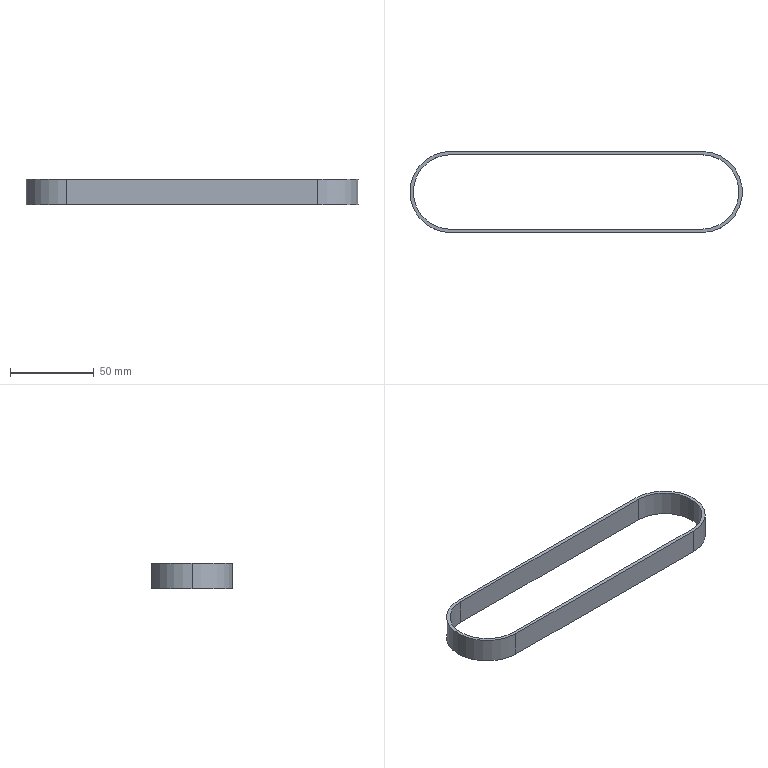Part | STEP file | J-ECP21-S5M-150-480 | 1 solid | 12 faces | box 198.56 x 48.56 x 15 mm | volume 13388 mm3 | cylinder 6 | plane 6 | commonest cylinder face diameters 44.56 x3 48.56 x3
STEP:
#1=CARTESIAN_POINT('',(0.,0.,0.));
#2=DIRECTION('',(0.,0.,1.));
#3=DIRECTION('',(1.,0.,0.));
#4=AXIS2_PLACEMENT_3D('',#1,#2,#3);
#5=CARTESIAN_POINT('',(0.,22.28,7.5));
#6=VERTEX_POINT('',#5);
#7=CARTESIAN_POINT('',(0.,22.28,-7.5));
#8=VERTEX_POINT('',#7);
#9=CARTESIAN_POINT('',(0.,22.28,7.5));
#10=DIRECTION('',(0.,0.,-1.));
#11=VECTOR('',#10,1.);
#12=LINE('',#9,#11);
#13=CARTESIAN_POINT('',(0.,0.,7.5));
#14=DIRECTION('',(0.,0.,-1.));
#15=DIRECTION('',(-1.,0.,0.));
#16=AXIS2_PLACEMENT_3D('',#13,#14,#15);
#17=CYLINDRICAL_SURFACE('',#16,22.28);
#18=CARTESIAN_POINT('',(1.571,0.));
#19=DIRECTION('',(0.,1.));
#20=VECTOR('',#19,1.);
#21=LINE('',#18,#20);
#22=(GEOMETRIC_REPRESENTATION_CONTEXT(2)PARAMETRIC_REPRESENTATION_CONTEXT()REPRESENTATION_CONTEXT('',''));
#23=DEFINITIONAL_REPRESENTATION('',(#21),#22);
#24=PCURVE('',#17,#23);
#25=CARTESIAN_POINT('',(0.,22.28,7.5));
#26=DIRECTION('',(0.,-1.,0.));
#27=DIRECTION('',(1.,0.,0.));
#28=AXIS2_PLACEMENT_3D('',#25,#26,#27);
#29=PLANE('',#28);
#30=CARTESIAN_POINT('',(0.,0.));
#31=DIRECTION('',(0.,-1.));
#32=VECTOR('',#31,1.);
#33=LINE('',#30,#32);
#34=(GEOMETRIC_REPRESENTATION_CONTEXT(2)PARAMETRIC_REPRESENTATION_CONTEXT()REPRESENTATION_CONTEXT('',''));
#35=DEFINITIONAL_REPRESENTATION('',(#33),#34);
#36=PCURVE('',#29,#35);
#37=SURFACE_CURVE('',#12,(#24,#36),.PCURVE_S1.);
#38=EDGE_CURVE('',#6,#8,#37,.T.);
#39=ORIENTED_EDGE('',*,*,#38,.T.);
#40=CARTESIAN_POINT('',(-22.28,0.,-7.5));
#41=VERTEX_POINT('',#40);
#42=CARTESIAN_POINT('',(0.,0.,-7.5));
#43=DIRECTION('',(0.,0.,1.));
#44=DIRECTION('',(1.,0.,0.));
#45=AXIS2_PLACEMENT_3D('',#42,#43,#44);
#46=CIRCLE('',#45,22.28);
#47=CARTESIAN_POINT('',(3.142,15.));
#48=DIRECTION('',(-1.,0.));
#49=VECTOR('',#48,1.);
#50=LINE('',#47,#49);
#51=(GEOMETRIC_REPRESENTATION_CONTEXT(2)PARAMETRIC_REPRESENTATION_CONTEXT()REPRESENTATION_CONTEXT('',''));
#52=DEFINITIONAL_REPRESENTATION('',(#50),#51);
#53=PCURVE('',#17,#52);
#54=CARTESIAN_POINT('',(0.,0.,-7.5));
#55=DIRECTION('',(0.,0.,1.));
#56=DIRECTION('',(1.,0.,0.));
#57=AXIS2_PLACEMENT_3D('',#54,#55,#56);
#58=PLANE('',#57);
#59=CARTESIAN_POINT('',(0.,0.));
#60=DIRECTION('',(1.,0.));
#61=AXIS2_PLACEMENT_2D('',#59,#60);
#62=CIRCLE('',#61,22.28);
#63=(GEOMETRIC_REPRESENTATION_CONTEXT(2)PARAMETRIC_REPRESENTATION_CONTEXT()REPRESENTATION_CONTEXT('',''));
#64=DEFINITIONAL_REPRESENTATION('',(#62),#63);
#65=PCURVE('',#58,#64);
#66=SURFACE_CURVE('',#46,(#53,#65),.PCURVE_S1.);
#67=EDGE_CURVE('',#8,#41,#66,.T.);
#68=ORIENTED_EDGE('',*,*,#67,.T.);
#69=CARTESIAN_POINT('',(-22.28,0.,7.5));
#70=VERTEX_POINT('',#69);
#71=CARTESIAN_POINT('',(-22.28,0.,7.5));
#72=DIRECTION('',(0.,0.,-1.));
#73=VECTOR('',#72,1.);
#74=LINE('',#71,#73);
#75=CARTESIAN_POINT('',(0.,0.));
#76=DIRECTION('',(0.,1.));
#77=VECTOR('',#76,1.);
#78=LINE('',#75,#77);
#79=(GEOMETRIC_REPRESENTATION_CONTEXT(2)PARAMETRIC_REPRESENTATION_CONTEXT()REPRESENTATION_CONTEXT('',''));
#80=DEFINITIONAL_REPRESENTATION('',(#78),#79);
#81=PCURVE('',#17,#80);
#82=CARTESIAN_POINT('',(0.,0.,7.5));
#83=DIRECTION('',(0.,0.,-1.));
#84=DIRECTION('',(-1.,0.,0.));
#85=AXIS2_PLACEMENT_3D('',#82,#83,#84);
#86=CYLINDRICAL_SURFACE('',#85,22.28);
#87=CARTESIAN_POINT('',(6.283,0.));
#88=DIRECTION('',(0.,1.));
#89=VECTOR('',#88,1.);
#90=LINE('',#87,#89);
#91=(GEOMETRIC_REPRESENTATION_CONTEXT(2)PARAMETRIC_REPRESENTATION_CONTEXT()REPRESENTATION_CONTEXT('',''));
#92=DEFINITIONAL_REPRESENTATION('',(#90),#91);
#93=PCURVE('',#86,#92);
#94=SURFACE_CURVE('',#74,(#81,#93),.PCURVE_S1.);
#95=EDGE_CURVE('',#70,#41,#94,.T.);
#96=ORIENTED_EDGE('',*,*,#95,.F.);
#97=CARTESIAN_POINT('',(0.,0.,7.5));
#98=DIRECTION('',(0.,0.,1.));
#99=DIRECTION('',(1.,0.,0.));
#100=AXIS2_PLACEMENT_3D('',#97,#98,#99);
#101=CIRCLE('',#100,22.28);
#102=CARTESIAN_POINT('',(3.142,0.));
#103=DIRECTION('',(-1.,0.));
#104=VECTOR('',#103,1.);
#105=LINE('',#102,#104);
#106=(GEOMETRIC_REPRESENTATION_CONTEXT(2)PARAMETRIC_REPRESENTATION_CONTEXT()REPRESENTATION_CONTEXT('',''));
#107=DEFINITIONAL_REPRESENTATION('',(#105),#106);
#108=PCURVE('',#17,#107);
#109=CARTESIAN_POINT('',(0.,0.,7.5));
#110=DIRECTION('',(0.,0.,1.));
#111=DIRECTION('',(1.,0.,0.));
#112=AXIS2_PLACEMENT_3D('',#109,#110,#111);
#113=PLANE('',#112);
#114=CARTESIAN_POINT('',(0.,0.));
#115=DIRECTION('',(1.,0.));
#116=AXIS2_PLACEMENT_2D('',#114,#115);
#117=CIRCLE('',#116,22.28);
#118=(GEOMETRIC_REPRESENTATION_CONTEXT(2)PARAMETRIC_REPRESENTATION_CONTEXT()REPRESENTATION_CONTEXT('',''));
#119=DEFINITIONAL_REPRESENTATION('',(#117),#118);
#120=PCURVE('',#113,#119);
#121=SURFACE_CURVE('',#101,(#108,#120),.PCURVE_S1.);
#122=EDGE_CURVE('',#6,#70,#121,.T.);
#123=ORIENTED_EDGE('',*,*,#122,.F.);
#124=EDGE_LOOP('',(#39,#68,#96,#123));
#125=FACE_BOUND('',#124,.F.);
#126=ADVANCED_FACE('',(#125),#17,.F.);
#127=CARTESIAN_POINT('',(-24.28,0.,7.5));
#128=VERTEX_POINT('',#127);
#129=CARTESIAN_POINT('',(0.,-24.28,7.5));
#130=VERTEX_POINT('',#129);
#131=CARTESIAN_POINT('',(0.,0.,7.5));
#132=DIRECTION('',(0.,0.,1.));
#133=DIRECTION('',(1.,0.,0.));
#134=AXIS2_PLACEMENT_3D('',#131,#132,#133);
#135=CIRCLE('',#134,24.28);
#136=CARTESIAN_POINT('',(0.,0.,7.5));
#137=DIRECTION('',(0.,0.,-1.));
#138=DIRECTION('',(-1.,0.,0.));
#139=AXIS2_PLACEMENT_3D('',#136,#137,#138);
#140=CYLINDRICAL_SURFACE('',#139,24.28);
#141=CARTESIAN_POINT('',(9.425,0.));
#142=DIRECTION('',(-1.,0.));
#143=VECTOR('',#142,1.);
#144=LINE('',#141,#143);
#145=(GEOMETRIC_REPRESENTATION_CONTEXT(2)PARAMETRIC_REPRESENTATION_CONTEXT()REPRESENTATION_CONTEXT('',''));
#146=DEFINITIONAL_REPRESENTATION('',(#144),#145);
#147=PCURVE('',#140,#146);
#148=CARTESIAN_POINT('',(0.,0.));
#149=DIRECTION('',(1.,0.));
#150=AXIS2_PLACEMENT_2D('',#148,#149);
#151=CIRCLE('',#150,24.28);
#152=(GEOMETRIC_REPRESENTATION_CONTEXT(2)PARAMETRIC_REPRESENTATION_CONTEXT()REPRESENTATION_CONTEXT('',''));
#153=DEFINITIONAL_REPRESENTATION('',(#151),#152);
#154=PCURVE('',#113,#153);
#155=SURFACE_CURVE('',#135,(#147,#154),.PCURVE_S1.);
#156=EDGE_CURVE('',#128,#130,#155,.T.);
#157=ORIENTED_EDGE('',*,*,#156,.F.);
#158=CARTESIAN_POINT('',(-24.28,0.,-7.5));
#159=VERTEX_POINT('',#158);
#160=CARTESIAN_POINT('',(-24.28,0.,7.5));
#161=DIRECTION('',(0.,0.,-1.));
#162=VECTOR('',#161,1.);
#163=LINE('',#160,#162);
#164=CARTESIAN_POINT('',(6.283,0.));
#165=DIRECTION('',(0.,1.));
#166=VECTOR('',#165,1.);
#167=LINE('',#164,#166);
#168=(GEOMETRIC_REPRESENTATION_CONTEXT(2)PARAMETRIC_REPRESENTATION_CONTEXT()REPRESENTATION_CONTEXT('',''));
#169=DEFINITIONAL_REPRESENTATION('',(#167),#168);
#170=PCURVE('',#140,#169);
#171=CARTESIAN_POINT('',(0.,0.,7.5));
#172=DIRECTION('',(0.,0.,-1.));
#173=DIRECTION('',(-1.,0.,0.));
#174=AXIS2_PLACEMENT_3D('',#171,#172,#173);
#175=CYLINDRICAL_SURFACE('',#174,24.28);
#176=CARTESIAN_POINT('',(0.,0.));
#177=DIRECTION('',(0.,1.));
#178=VECTOR('',#177,1.);
#179=LINE('',#176,#178);
#180=(GEOMETRIC_REPRESENTATION_CONTEXT(2)PARAMETRIC_REPRESENTATION_CONTEXT()REPRESENTATION_CONTEXT('',''));
#181=DEFINITIONAL_REPRESENTATION('',(#179),#180);
#182=PCURVE('',#175,#181);
#183=SURFACE_CURVE('',#163,(#170,#182),.PCURVE_S1.);
#184=EDGE_CURVE('',#128,#159,#183,.T.);
#185=ORIENTED_EDGE('',*,*,#184,.T.);
#186=CARTESIAN_POINT('',(0.,-24.28,-7.5));
#187=VERTEX_POINT('',#186);
#188=CARTESIAN_POINT('',(0.,0.,-7.5));
#189=DIRECTION('',(0.,0.,1.));
#190=DIRECTION('',(1.,0.,0.));
#191=AXIS2_PLACEMENT_3D('',#188,#189,#190);
#192=CIRCLE('',#191,24.28);
#193=CARTESIAN_POINT('',(9.425,15.));
#194=DIRECTION('',(-1.,0.));
#195=VECTOR('',#194,1.);
#196=LINE('',#193,#195);
#197=(GEOMETRIC_REPRESENTATION_CONTEXT(2)PARAMETRIC_REPRESENTATION_CONTEXT()REPRESENTATION_CONTEXT('',''));
#198=DEFINITIONAL_REPRESENTATION('',(#196),#197);
#199=PCURVE('',#140,#198);
#200=CARTESIAN_POINT('',(0.,0.));
#201=DIRECTION('',(1.,0.));
#202=AXIS2_PLACEMENT_2D('',#200,#201);
#203=CIRCLE('',#202,24.28);
#204=(GEOMETRIC_REPRESENTATION_CONTEXT(2)PARAMETRIC_REPRESENTATION_CONTEXT()REPRESENTATION_CONTEXT('',''));
#205=DEFINITIONAL_REPRESENTATION('',(#203),#204);
#206=PCURVE('',#58,#205);
#207=SURFACE_CURVE('',#192,(#199,#206),.PCURVE_S1.);
#208=EDGE_CURVE('',#159,#187,#207,.T.);
#209=ORIENTED_EDGE('',*,*,#208,.T.);
#210=CARTESIAN_POINT('',(0.,-24.28,7.5));
#211=DIRECTION('',(0.,0.,-1.));
#212=VECTOR('',#211,1.);
#213=LINE('',#210,#212);
#214=CARTESIAN_POINT('',(4.712,0.));
#215=DIRECTION('',(0.,1.));
#216=VECTOR('',#215,1.);
#217=LINE('',#214,#216);
#218=(GEOMETRIC_REPRESENTATION_CONTEXT(2)PARAMETRIC_REPRESENTATION_CONTEXT()REPRESENTATION_CONTEXT('',''));
#219=DEFINITIONAL_REPRESENTATION('',(#217),#218);
#220=PCURVE('',#140,#219);
#221=CARTESIAN_POINT('',(150.,-24.28,7.5));
#222=DIRECTION('',(0.,1.,0.));
#223=DIRECTION('',(-1.,0.,0.));
#224=AXIS2_PLACEMENT_3D('',#221,#222,#223);
#225=PLANE('',#224);
#226=CARTESIAN_POINT('',(150.,0.));
#227=DIRECTION('',(0.,-1.));
#228=VECTOR('',#227,1.);
#229=LINE('',#226,#228);
#230=(GEOMETRIC_REPRESENTATION_CONTEXT(2)PARAMETRIC_REPRESENTATION_CONTEXT()REPRESENTATION_CONTEXT('',''));
#231=DEFINITIONAL_REPRESENTATION('',(#229),#230);
#232=PCURVE('',#225,#231);
#233=SURFACE_CURVE('',#213,(#220,#232),.PCURVE_S1.);
#234=EDGE_CURVE('',#130,#187,#233,.T.);
#235=ORIENTED_EDGE('',*,*,#234,.F.);
#236=EDGE_LOOP('',(#157,#185,#209,#235));
#237=FACE_BOUND('',#236,.T.);
#238=ADVANCED_FACE('',(#237),#140,.T.);
#239=CARTESIAN_POINT('',(0.,24.28,7.5));
#240=VERTEX_POINT('',#239);
#241=CARTESIAN_POINT('',(0.,0.,7.5));
#242=DIRECTION('',(0.,0.,1.));
#243=DIRECTION('',(1.,0.,0.));
#244=AXIS2_PLACEMENT_3D('',#241,#242,#243);
#245=CIRCLE('',#244,24.28);
#246=CARTESIAN_POINT('',(0.,0.));
#247=DIRECTION('',(1.,0.));
#248=AXIS2_PLACEMENT_2D('',#246,#247);
#249=CIRCLE('',#248,24.28);
#250=(GEOMETRIC_REPRESENTATION_CONTEXT(2)PARAMETRIC_REPRESENTATION_CONTEXT()REPRESENTATION_CONTEXT('',''));
#251=DEFINITIONAL_REPRESENTATION('',(#249),#250);
#252=PCURVE('',#113,#251);
#253=CARTESIAN_POINT('',(3.142,0.));
#254=DIRECTION('',(-1.,0.));
#255=VECTOR('',#254,1.);
#256=LINE('',#253,#255);
#257=(GEOMETRIC_REPRESENTATION_CONTEXT(2)PARAMETRIC_REPRESENTATION_CONTEXT()REPRESENTATION_CONTEXT('',''));
#258=DEFINITIONAL_REPRESENTATION('',(#256),#257);
#259=PCURVE('',#175,#258);
#260=SURFACE_CURVE('',#245,(#252,#259),.PCURVE_S1.);
#261=EDGE_CURVE('',#240,#128,#260,.T.);
#262=ORIENTED_EDGE('',*,*,#261,.T.);
#263=ORIENTED_EDGE('',*,*,#156,.T.);
#264=CARTESIAN_POINT('',(150.,-24.28,7.5));
#265=VERTEX_POINT('',#264);
#266=CARTESIAN_POINT('',(150.,-24.28,7.5));
#267=DIRECTION('',(1.,0.,0.));
#268=VECTOR('',#267,1.);
#269=LINE('',#266,#268);
#270=CARTESIAN_POINT('',(150.,-24.28));
#271=DIRECTION('',(1.,0.));
#272=VECTOR('',#271,1.);
#273=LINE('',#270,#272);
#274=(GEOMETRIC_REPRESENTATION_CONTEXT(2)PARAMETRIC_REPRESENTATION_CONTEXT()REPRESENTATION_CONTEXT('',''));
#275=DEFINITIONAL_REPRESENTATION('',(#273),#274);
#276=PCURVE('',#113,#275);
#277=CARTESIAN_POINT('',(0.,0.));
#278=DIRECTION('',(-1.,0.));
#279=VECTOR('',#278,1.);
#280=LINE('',#277,#279);
#281=(GEOMETRIC_REPRESENTATION_CONTEXT(2)PARAMETRIC_REPRESENTATION_CONTEXT()REPRESENTATION_CONTEXT('',''));
#282=DEFINITIONAL_REPRESENTATION('',(#280),#281);
#283=PCURVE('',#225,#282);
#284=SURFACE_CURVE('',#269,(#276,#283),.PCURVE_S1.);
#285=EDGE_CURVE('',#130,#265,#284,.T.);
#286=ORIENTED_EDGE('',*,*,#285,.T.);
#287=CARTESIAN_POINT('',(150.,24.28,7.5));
#288=VERTEX_POINT('',#287);
#289=CARTESIAN_POINT('',(150.,0.,7.5));
#290=DIRECTION('',(0.,0.,1.));
#291=DIRECTION('',(1.,0.,0.));
#292=AXIS2_PLACEMENT_3D('',#289,#290,#291);
#293=CIRCLE('',#292,24.28);
#294=CARTESIAN_POINT('',(150.,0.));
#295=DIRECTION('',(1.,0.));
#296=AXIS2_PLACEMENT_2D('',#294,#295);
#297=CIRCLE('',#296,24.28);
#298=(GEOMETRIC_REPRESENTATION_CONTEXT(2)PARAMETRIC_REPRESENTATION_CONTEXT()REPRESENTATION_CONTEXT('',''));
#299=DEFINITIONAL_REPRESENTATION('',(#297),#298);
#300=PCURVE('',#113,#299);
#301=CARTESIAN_POINT('',(150.,0.,7.5));
#302=DIRECTION('',(0.,0.,-1.));
#303=DIRECTION('',(-1.,0.,0.));
#304=AXIS2_PLACEMENT_3D('',#301,#302,#303);
#305=CYLINDRICAL_SURFACE('',#304,24.28);
#306=CARTESIAN_POINT('',(9.425,0.));
#307=DIRECTION('',(-1.,0.));
#308=VECTOR('',#307,1.);
#309=LINE('',#306,#308);
#310=(GEOMETRIC_REPRESENTATION_CONTEXT(2)PARAMETRIC_REPRESENTATION_CONTEXT()REPRESENTATION_CONTEXT('',''));
#311=DEFINITIONAL_REPRESENTATION('',(#309),#310);
#312=PCURVE('',#305,#311);
#313=SURFACE_CURVE('',#293,(#300,#312),.PCURVE_S1.);
#314=EDGE_CURVE('',#265,#288,#313,.T.);
#315=ORIENTED_EDGE('',*,*,#314,.T.);
#316=CARTESIAN_POINT('',(0.,24.28,7.5));
#317=DIRECTION('',(-1.,0.,0.));
#318=VECTOR('',#317,1.);
#319=LINE('',#316,#318);
#320=CARTESIAN_POINT('',(0.,24.28));
#321=DIRECTION('',(-1.,0.));
#322=VECTOR('',#321,1.);
#323=LINE('',#320,#322);
#324=(GEOMETRIC_REPRESENTATION_CONTEXT(2)PARAMETRIC_REPRESENTATION_CONTEXT()REPRESENTATION_CONTEXT('',''));
#325=DEFINITIONAL_REPRESENTATION('',(#323),#324);
#326=PCURVE('',#113,#325);
#327=CARTESIAN_POINT('',(0.,24.28,7.5));
#328=DIRECTION('',(0.,-1.,0.));
#329=DIRECTION('',(1.,0.,0.));
#330=AXIS2_PLACEMENT_3D('',#327,#328,#329);
#331=PLANE('',#330);
#332=CARTESIAN_POINT('',(0.,0.));
#333=DIRECTION('',(-1.,0.));
#334=VECTOR('',#333,1.);
#335=LINE('',#332,#334);
#336=(GEOMETRIC_REPRESENTATION_CONTEXT(2)PARAMETRIC_REPRESENTATION_CONTEXT()REPRESENTATION_CONTEXT('',''));
#337=DEFINITIONAL_REPRESENTATION('',(#335),#336);
#338=PCURVE('',#331,#337);
#339=SURFACE_CURVE('',#319,(#326,#338),.PCURVE_S1.);
#340=EDGE_CURVE('',#288,#240,#339,.T.);
#341=ORIENTED_EDGE('',*,*,#340,.T.);
#342=EDGE_LOOP('',(#262,#263,#286,#315,#341));
#343=FACE_BOUND('',#342,.T.);
#344=CARTESIAN_POINT('',(0.,-22.28,7.5));
#345=VERTEX_POINT('',#344);
#346=CARTESIAN_POINT('',(150.,-22.28,7.5));
#347=VERTEX_POINT('',#346);
#348=CARTESIAN_POINT('',(150.,-22.28,7.5));
#349=DIRECTION('',(1.,0.,0.));
#350=VECTOR('',#349,1.);
#351=LINE('',#348,#350);
#352=CARTESIAN_POINT('',(150.,-22.28));
#353=DIRECTION('',(1.,0.));
#354=VECTOR('',#353,1.);
#355=LINE('',#352,#354);
#356=(GEOMETRIC_REPRESENTATION_CONTEXT(2)PARAMETRIC_REPRESENTATION_CONTEXT()REPRESENTATION_CONTEXT('',''));
#357=DEFINITIONAL_REPRESENTATION('',(#355),#356);
#358=PCURVE('',#113,#357);
#359=CARTESIAN_POINT('',(150.,-22.28,7.5));
#360=DIRECTION('',(0.,1.,0.));
#361=DIRECTION('',(-1.,0.,0.));
#362=AXIS2_PLACEMENT_3D('',#359,#360,#361);
#363=PLANE('',#362);
#364=CARTESIAN_POINT('',(0.,0.));
#365=DIRECTION('',(-1.,0.));
#366=VECTOR('',#365,1.);
#367=LINE('',#364,#366);
#368=(GEOMETRIC_REPRESENTATION_CONTEXT(2)PARAMETRIC_REPRESENTATION_CONTEXT()REPRESENTATION_CONTEXT('',''));
#369=DEFINITIONAL_REPRESENTATION('',(#367),#368);
#370=PCURVE('',#363,#369);
#371=SURFACE_CURVE('',#351,(#358,#370),.PCURVE_S1.);
#372=EDGE_CURVE('',#345,#347,#371,.T.);
#373=ORIENTED_EDGE('',*,*,#372,.F.);
#374=CARTESIAN_POINT('',(0.,0.,7.5));
#375=DIRECTION('',(0.,0.,1.));
#376=DIRECTION('',(1.,0.,0.));
#377=AXIS2_PLACEMENT_3D('',#374,#375,#376);
#378=CIRCLE('',#377,22.28);
#379=CARTESIAN_POINT('',(0.,0.));
#380=DIRECTION('',(1.,0.));
#381=AXIS2_PLACEMENT_2D('',#379,#380);
#382=CIRCLE('',#381,22.28);
#383=(GEOMETRIC_REPRESENTATION_CONTEXT(2)PARAMETRIC_REPRESENTATION_CONTEXT()REPRESENTATION_CONTEXT('',''));
#384=DEFINITIONAL_REPRESENTATION('',(#382),#383);
#385=PCURVE('',#113,#384);
#386=CARTESIAN_POINT('',(9.425,0.));
#387=DIRECTION('',(-1.,0.));
#388=VECTOR('',#387,1.);
#389=LINE('',#386,#388);
#390=(GEOMETRIC_REPRESENTATION_CONTEXT(2)PARAMETRIC_REPRESENTATION_CONTEXT()REPRESENTATION_CONTEXT('',''));
#391=DEFINITIONAL_REPRESENTATION('',(#389),#390);
#392=PCURVE('',#86,#391);
#393=SURFACE_CURVE('',#378,(#385,#392),.PCURVE_S1.);
#394=EDGE_CURVE('',#70,#345,#393,.T.);
#395=ORIENTED_EDGE('',*,*,#394,.F.);
#396=ORIENTED_EDGE('',*,*,#122,.F.);
#397=CARTESIAN_POINT('',(150.,22.28,7.5));
#398=VERTEX_POINT('',#397);
#399=CARTESIAN_POINT('',(0.,22.28,7.5));
#400=DIRECTION('',(-1.,0.,0.));
#401=VECTOR('',#400,1.);
#402=LINE('',#399,#401);
#403=CARTESIAN_POINT('',(0.,22.28));
#404=DIRECTION('',(-1.,0.));
#405=VECTOR('',#404,1.);
#406=LINE('',#403,#405);
#407=(GEOMETRIC_REPRESENTATION_CONTEXT(2)PARAMETRIC_REPRESENTATION_CONTEXT()REPRESENTATION_CONTEXT('',''));
#408=DEFINITIONAL_REPRESENTATION('',(#406),#407);
#409=PCURVE('',#113,#408);
#410=CARTESIAN_POINT('',(0.,0.));
#411=DIRECTION('',(-1.,0.));
#412=VECTOR('',#411,1.);
#413=LINE('',#410,#412);
#414=(GEOMETRIC_REPRESENTATION_CONTEXT(2)PARAMETRIC_REPRESENTATION_CONTEXT()REPRESENTATION_CONTEXT('',''));
#415=DEFINITIONAL_REPRESENTATION('',(#413),#414);
#416=PCURVE('',#29,#415);
#417=SURFACE_CURVE('',#402,(#409,#416),.PCURVE_S1.);
#418=EDGE_CURVE('',#398,#6,#417,.T.);
#419=ORIENTED_EDGE('',*,*,#418,.F.);
#420=CARTESIAN_POINT('',(150.,0.,7.5));
#421=DIRECTION('',(0.,0.,1.));
#422=DIRECTION('',(1.,0.,0.));
#423=AXIS2_PLACEMENT_3D('',#420,#421,#422);
#424=CIRCLE('',#423,22.28);
#425=CARTESIAN_POINT('',(150.,0.));
#426=DIRECTION('',(1.,0.));
#427=AXIS2_PLACEMENT_2D('',#425,#426);
#428=CIRCLE('',#427,22.28);
#429=(GEOMETRIC_REPRESENTATION_CONTEXT(2)PARAMETRIC_REPRESENTATION_CONTEXT()REPRESENTATION_CONTEXT('',''));
#430=DEFINITIONAL_REPRESENTATION('',(#428),#429);
#431=PCURVE('',#113,#430);
#432=CARTESIAN_POINT('',(150.,0.,7.5));
#433=DIRECTION('',(0.,0.,-1.));
#434=DIRECTION('',(-1.,0.,0.));
#435=AXIS2_PLACEMENT_3D('',#432,#433,#434);
#436=CYLINDRICAL_SURFACE('',#435,22.28);
#437=CARTESIAN_POINT('',(9.425,0.));
#438=DIRECTION('',(-1.,0.));
#439=VECTOR('',#438,1.);
#440=LINE('',#437,#439);
#441=(GEOMETRIC_REPRESENTATION_CONTEXT(2)PARAMETRIC_REPRESENTATION_CONTEXT()REPRESENTATION_CONTEXT('',''));
#442=DEFINITIONAL_REPRESENTATION('',(#440),#441);
#443=PCURVE('',#436,#442);
#444=SURFACE_CURVE('',#424,(#431,#443),.PCURVE_S1.);
#445=EDGE_CURVE('',#347,#398,#444,.T.);
#446=ORIENTED_EDGE('',*,*,#445,.F.);
#447=EDGE_LOOP('',(#373,#395,#396,#419,#446));
#448=FACE_BOUND('',#447,.T.);
#449=ADVANCED_FACE('',(#343,#448),#113,.T.);
#450=CARTESIAN_POINT('',(0.,24.28,-7.5));
#451=VERTEX_POINT('',#450);
#452=CARTESIAN_POINT('',(0.,0.,-7.5));
#453=DIRECTION('',(0.,0.,1.));
#454=DIRECTION('',(1.,0.,0.));
#455=AXIS2_PLACEMENT_3D('',#452,#453,#454);
#456=CIRCLE('',#455,24.28);
#457=CARTESIAN_POINT('',(0.,0.));
#458=DIRECTION('',(1.,0.));
#459=AXIS2_PLACEMENT_2D('',#457,#458);
#460=CIRCLE('',#459,24.28);
#461=(GEOMETRIC_REPRESENTATION_CONTEXT(2)PARAMETRIC_REPRESENTATION_CONTEXT()REPRESENTATION_CONTEXT('',''));
#462=DEFINITIONAL_REPRESENTATION('',(#460),#461);
#463=PCURVE('',#58,#462);
#464=CARTESIAN_POINT('',(3.142,15.));
#465=DIRECTION('',(-1.,0.));
#466=VECTOR('',#465,1.);
#467=LINE('',#464,#466);
#468=(GEOMETRIC_REPRESENTATION_CONTEXT(2)PARAMETRIC_REPRESENTATION_CONTEXT()REPRESENTATION_CONTEXT('',''));
#469=DEFINITIONAL_REPRESENTATION('',(#467),#468);
#470=PCURVE('',#175,#469);
#471=SURFACE_CURVE('',#456,(#463,#470),.PCURVE_S1.);
#472=EDGE_CURVE('',#451,#159,#471,.T.);
#473=ORIENTED_EDGE('',*,*,#472,.F.);
#474=CARTESIAN_POINT('',(150.,24.28,-7.5));
#475=VERTEX_POINT('',#474);
#476=CARTESIAN_POINT('',(0.,24.28,-7.5));
#477=DIRECTION('',(-1.,0.,0.));
#478=VECTOR('',#477,1.);
#479=LINE('',#476,#478);
#480=CARTESIAN_POINT('',(0.,24.28));
#481=DIRECTION('',(-1.,0.));
#482=VECTOR('',#481,1.);
#483=LINE('',#480,#482);
#484=(GEOMETRIC_REPRESENTATION_CONTEXT(2)PARAMETRIC_REPRESENTATION_CONTEXT()REPRESENTATION_CONTEXT('',''));
#485=DEFINITIONAL_REPRESENTATION('',(#483),#484);
#486=PCURVE('',#58,#485);
#487=CARTESIAN_POINT('',(0.,-15.));
#488=DIRECTION('',(-1.,0.));
#489=VECTOR('',#488,1.);
#490=LINE('',#487,#489);
#491=(GEOMETRIC_REPRESENTATION_CONTEXT(2)PARAMETRIC_REPRESENTATION_CONTEXT()REPRESENTATION_CONTEXT('',''));
#492=DEFINITIONAL_REPRESENTATION('',(#490),#491);
#493=PCURVE('',#331,#492);
#494=SURFACE_CURVE('',#479,(#486,#493),.PCURVE_S1.);
#495=EDGE_CURVE('',#475,#451,#494,.T.);
#496=ORIENTED_EDGE('',*,*,#495,.F.);
#497=CARTESIAN_POINT('',(150.,-24.28,-7.5));
#498=VERTEX_POINT('',#497);
#499=CARTESIAN_POINT('',(150.,0.,-7.5));
#500=DIRECTION('',(0.,0.,1.));
#501=DIRECTION('',(1.,0.,0.));
#502=AXIS2_PLACEMENT_3D('',#499,#500,#501);
#503=CIRCLE('',#502,24.28);
#504=CARTESIAN_POINT('',(150.,0.));
#505=DIRECTION('',(1.,0.));
#506=AXIS2_PLACEMENT_2D('',#504,#505);
#507=CIRCLE('',#506,24.28);
#508=(GEOMETRIC_REPRESENTATION_CONTEXT(2)PARAMETRIC_REPRESENTATION_CONTEXT()REPRESENTATION_CONTEXT('',''));
#509=DEFINITIONAL_REPRESENTATION('',(#507),#508);
#510=PCURVE('',#58,#509);
#511=CARTESIAN_POINT('',(9.425,15.));
#512=DIRECTION('',(-1.,0.));
#513=VECTOR('',#512,1.);
#514=LINE('',#511,#513);
#515=(GEOMETRIC_REPRESENTATION_CONTEXT(2)PARAMETRIC_REPRESENTATION_CONTEXT()REPRESENTATION_CONTEXT('',''));
#516=DEFINITIONAL_REPRESENTATION('',(#514),#515);
#517=PCURVE('',#305,#516);
#518=SURFACE_CURVE('',#503,(#510,#517),.PCURVE_S1.);
#519=EDGE_CURVE('',#498,#475,#518,.T.);
#520=ORIENTED_EDGE('',*,*,#519,.F.);
#521=CARTESIAN_POINT('',(150.,-24.28,-7.5));
#522=DIRECTION('',(1.,0.,0.));
#523=VECTOR('',#522,1.);
#524=LINE('',#521,#523);
#525=CARTESIAN_POINT('',(150.,-24.28));
#526=DIRECTION('',(1.,0.));
#527=VECTOR('',#526,1.);
#528=LINE('',#525,#527);
#529=(GEOMETRIC_REPRESENTATION_CONTEXT(2)PARAMETRIC_REPRESENTATION_CONTEXT()REPRESENTATION_CONTEXT('',''));
#530=DEFINITIONAL_REPRESENTATION('',(#528),#529);
#531=PCURVE('',#58,#530);
#532=CARTESIAN_POINT('',(0.,-15.));
#533=DIRECTION('',(-1.,0.));
#534=VECTOR('',#533,1.);
#535=LINE('',#532,#534);
#536=(GEOMETRIC_REPRESENTATION_CONTEXT(2)PARAMETRIC_REPRESENTATION_CONTEXT()REPRESENTATION_CONTEXT('',''));
#537=DEFINITIONAL_REPRESENTATION('',(#535),#536);
#538=PCURVE('',#225,#537);
#539=SURFACE_CURVE('',#524,(#531,#538),.PCURVE_S1.);
#540=EDGE_CURVE('',#187,#498,#539,.T.);
#541=ORIENTED_EDGE('',*,*,#540,.F.);
#542=ORIENTED_EDGE('',*,*,#208,.F.);
#543=EDGE_LOOP('',(#473,#496,#520,#541,#542));
#544=FACE_BOUND('',#543,.T.);
#545=ORIENTED_EDGE('',*,*,#67,.T.);
#546=CARTESIAN_POINT('',(0.,-22.28,-7.5));
#547=VERTEX_POINT('',#546);
#548=CARTESIAN_POINT('',(0.,0.,-7.5));
#549=DIRECTION('',(0.,0.,1.));
#550=DIRECTION('',(1.,0.,0.));
#551=AXIS2_PLACEMENT_3D('',#548,#549,#550);
#552=CIRCLE('',#551,22.28);
#553=CARTESIAN_POINT('',(0.,0.));
#554=DIRECTION('',(1.,0.));
#555=AXIS2_PLACEMENT_2D('',#553,#554);
#556=CIRCLE('',#555,22.28);
#557=(GEOMETRIC_REPRESENTATION_CONTEXT(2)PARAMETRIC_REPRESENTATION_CONTEXT()REPRESENTATION_CONTEXT('',''));
#558=DEFINITIONAL_REPRESENTATION('',(#556),#557);
#559=PCURVE('',#58,#558);
#560=CARTESIAN_POINT('',(9.425,15.));
#561=DIRECTION('',(-1.,0.));
#562=VECTOR('',#561,1.);
#563=LINE('',#560,#562);
#564=(GEOMETRIC_REPRESENTATION_CONTEXT(2)PARAMETRIC_REPRESENTATION_CONTEXT()REPRESENTATION_CONTEXT('',''));
#565=DEFINITIONAL_REPRESENTATION('',(#563),#564);
#566=PCURVE('',#86,#565);
#567=SURFACE_CURVE('',#552,(#559,#566),.PCURVE_S1.);
#568=EDGE_CURVE('',#41,#547,#567,.T.);
#569=ORIENTED_EDGE('',*,*,#568,.T.);
#570=CARTESIAN_POINT('',(150.,-22.28,-7.5));
#571=VERTEX_POINT('',#570);
#572=CARTESIAN_POINT('',(150.,-22.28,-7.5));
#573=DIRECTION('',(1.,0.,0.));
#574=VECTOR('',#573,1.);
#575=LINE('',#572,#574);
#576=CARTESIAN_POINT('',(150.,-22.28));
#577=DIRECTION('',(1.,0.));
#578=VECTOR('',#577,1.);
#579=LINE('',#576,#578);
#580=(GEOMETRIC_REPRESENTATION_CONTEXT(2)PARAMETRIC_REPRESENTATION_CONTEXT()REPRESENTATION_CONTEXT('',''));
#581=DEFINITIONAL_REPRESENTATION('',(#579),#580);
#582=PCURVE('',#58,#581);
#583=CARTESIAN_POINT('',(0.,-15.));
#584=DIRECTION('',(-1.,0.));
#585=VECTOR('',#584,1.);
#586=LINE('',#583,#585);
#587=(GEOMETRIC_REPRESENTATION_CONTEXT(2)PARAMETRIC_REPRESENTATION_CONTEXT()REPRESENTATION_CONTEXT('',''));
#588=DEFINITIONAL_REPRESENTATION('',(#586),#587);
#589=PCURVE('',#363,#588);
#590=SURFACE_CURVE('',#575,(#582,#589),.PCURVE_S1.);
#591=EDGE_CURVE('',#547,#571,#590,.T.);
#592=ORIENTED_EDGE('',*,*,#591,.T.);
#593=CARTESIAN_POINT('',(150.,22.28,-7.5));
#594=VERTEX_POINT('',#593);
#595=CARTESIAN_POINT('',(150.,0.,-7.5));
#596=DIRECTION('',(0.,0.,1.));
#597=DIRECTION('',(1.,0.,0.));
#598=AXIS2_PLACEMENT_3D('',#595,#596,#597);
#599=CIRCLE('',#598,22.28);
#600=CARTESIAN_POINT('',(150.,0.));
#601=DIRECTION('',(1.,0.));
#602=AXIS2_PLACEMENT_2D('',#600,#601);
#603=CIRCLE('',#602,22.28);
#604=(GEOMETRIC_REPRESENTATION_CONTEXT(2)PARAMETRIC_REPRESENTATION_CONTEXT()REPRESENTATION_CONTEXT('',''));
#605=DEFINITIONAL_REPRESENTATION('',(#603),#604);
#606=PCURVE('',#58,#605);
#607=CARTESIAN_POINT('',(9.425,15.));
#608=DIRECTION('',(-1.,0.));
#609=VECTOR('',#608,1.);
#610=LINE('',#607,#609);
#611=(GEOMETRIC_REPRESENTATION_CONTEXT(2)PARAMETRIC_REPRESENTATION_CONTEXT()REPRESENTATION_CONTEXT('',''));
#612=DEFINITIONAL_REPRESENTATION('',(#610),#611);
#613=PCURVE('',#436,#612);
#614=SURFACE_CURVE('',#599,(#606,#613),.PCURVE_S1.);
#615=EDGE_CURVE('',#571,#594,#614,.T.);
#616=ORIENTED_EDGE('',*,*,#615,.T.);
#617=CARTESIAN_POINT('',(0.,22.28,-7.5));
#618=DIRECTION('',(-1.,0.,0.));
#619=VECTOR('',#618,1.);
#620=LINE('',#617,#619);
#621=CARTESIAN_POINT('',(0.,22.28));
#622=DIRECTION('',(-1.,0.));
#623=VECTOR('',#622,1.);
#624=LINE('',#621,#623);
#625=(GEOMETRIC_REPRESENTATION_CONTEXT(2)PARAMETRIC_REPRESENTATION_CONTEXT()REPRESENTATION_CONTEXT('',''));
#626=DEFINITIONAL_REPRESENTATION('',(#624),#625);
#627=PCURVE('',#58,#626);
#628=CARTESIAN_POINT('',(0.,-15.));
#629=DIRECTION('',(-1.,0.));
#630=VECTOR('',#629,1.);
#631=LINE('',#628,#630);
#632=(GEOMETRIC_REPRESENTATION_CONTEXT(2)PARAMETRIC_REPRESENTATION_CONTEXT()REPRESENTATION_CONTEXT('',''));
#633=DEFINITIONAL_REPRESENTATION('',(#631),#632);
#634=PCURVE('',#29,#633);
#635=SURFACE_CURVE('',#620,(#627,#634),.PCURVE_S1.);
#636=EDGE_CURVE('',#594,#8,#635,.T.);
#637=ORIENTED_EDGE('',*,*,#636,.T.);
#638=EDGE_LOOP('',(#545,#569,#592,#616,#637));
#639=FACE_BOUND('',#638,.T.);
#640=ADVANCED_FACE('',(#544,#639),#58,.F.);
#641=ORIENTED_EDGE('',*,*,#184,.F.);
#642=ORIENTED_EDGE('',*,*,#261,.F.);
#643=CARTESIAN_POINT('',(0.,24.28,7.5));
#644=DIRECTION('',(0.,0.,-1.));
#645=VECTOR('',#644,1.);
#646=LINE('',#643,#645);
#647=CARTESIAN_POINT('',(1.571,0.));
#648=DIRECTION('',(0.,1.));
#649=VECTOR('',#648,1.);
#650=LINE('',#647,#649);
#651=(GEOMETRIC_REPRESENTATION_CONTEXT(2)PARAMETRIC_REPRESENTATION_CONTEXT()REPRESENTATION_CONTEXT('',''));
#652=DEFINITIONAL_REPRESENTATION('',(#650),#651);
#653=PCURVE('',#175,#652);
#654=CARTESIAN_POINT('',(0.,0.));
#655=DIRECTION('',(0.,-1.));
#656=VECTOR('',#655,1.);
#657=LINE('',#654,#656);
#658=(GEOMETRIC_REPRESENTATION_CONTEXT(2)PARAMETRIC_REPRESENTATION_CONTEXT()REPRESENTATION_CONTEXT('',''));
#659=DEFINITIONAL_REPRESENTATION('',(#657),#658);
#660=PCURVE('',#331,#659);
#661=SURFACE_CURVE('',#646,(#653,#660),.PCURVE_S1.);
#662=EDGE_CURVE('',#240,#451,#661,.T.);
#663=ORIENTED_EDGE('',*,*,#662,.T.);
#664=ORIENTED_EDGE('',*,*,#472,.T.);
#665=EDGE_LOOP('',(#641,#642,#663,#664));
#666=FACE_BOUND('',#665,.T.);
#667=ADVANCED_FACE('',(#666),#175,.T.);
#668=ORIENTED_EDGE('',*,*,#540,.T.);
#669=CARTESIAN_POINT('',(150.,-24.28,7.5));
#670=DIRECTION('',(0.,0.,-1.));
#671=VECTOR('',#670,1.);
#672=LINE('',#669,#671);
#673=CARTESIAN_POINT('',(0.,0.));
#674=DIRECTION('',(0.,-1.));
#675=VECTOR('',#674,1.);
#676=LINE('',#673,#675);
#677=(GEOMETRIC_REPRESENTATION_CONTEXT(2)PARAMETRIC_REPRESENTATION_CONTEXT()REPRESENTATION_CONTEXT('',''));
#678=DEFINITIONAL_REPRESENTATION('',(#676),#677);
#679=PCURVE('',#225,#678);
#680=CARTESIAN_POINT('',(4.712,0.));
#681=DIRECTION('',(0.,1.));
#682=VECTOR('',#681,1.);
#683=LINE('',#680,#682);
#684=(GEOMETRIC_REPRESENTATION_CONTEXT(2)PARAMETRIC_REPRESENTATION_CONTEXT()REPRESENTATION_CONTEXT('',''));
#685=DEFINITIONAL_REPRESENTATION('',(#683),#684);
#686=PCURVE('',#305,#685);
#687=SURFACE_CURVE('',#672,(#679,#686),.PCURVE_S1.);
#688=EDGE_CURVE('',#265,#498,#687,.T.);
#689=ORIENTED_EDGE('',*,*,#688,.F.);
#690=ORIENTED_EDGE('',*,*,#285,.F.);
#691=ORIENTED_EDGE('',*,*,#234,.T.);
#692=EDGE_LOOP('',(#668,#689,#690,#691));
#693=FACE_BOUND('',#692,.T.);
#694=ADVANCED_FACE('',(#693),#225,.F.);
#695=ORIENTED_EDGE('',*,*,#519,.T.);
#696=CARTESIAN_POINT('',(150.,24.28,7.5));
#697=DIRECTION('',(0.,0.,-1.));
#698=VECTOR('',#697,1.);
#699=LINE('',#696,#698);
#700=CARTESIAN_POINT('',(1.571,0.));
#701=DIRECTION('',(0.,1.));
#702=VECTOR('',#701,1.);
#703=LINE('',#700,#702);
#704=(GEOMETRIC_REPRESENTATION_CONTEXT(2)PARAMETRIC_REPRESENTATION_CONTEXT()REPRESENTATION_CONTEXT('',''));
#705=DEFINITIONAL_REPRESENTATION('',(#703),#704);
#706=PCURVE('',#305,#705);
#707=CARTESIAN_POINT('',(150.,0.));
#708=DIRECTION('',(0.,-1.));
#709=VECTOR('',#708,1.);
#710=LINE('',#707,#709);
#711=(GEOMETRIC_REPRESENTATION_CONTEXT(2)PARAMETRIC_REPRESENTATION_CONTEXT()REPRESENTATION_CONTEXT('',''));
#712=DEFINITIONAL_REPRESENTATION('',(#710),#711);
#713=PCURVE('',#331,#712);
#714=SURFACE_CURVE('',#699,(#706,#713),.PCURVE_S1.);
#715=EDGE_CURVE('',#288,#475,#714,.T.);
#716=ORIENTED_EDGE('',*,*,#715,.F.);
#717=ORIENTED_EDGE('',*,*,#314,.F.);
#718=ORIENTED_EDGE('',*,*,#688,.T.);
#719=EDGE_LOOP('',(#695,#716,#717,#718));
#720=FACE_BOUND('',#719,.T.);
#721=ADVANCED_FACE('',(#720),#305,.T.);
#722=ORIENTED_EDGE('',*,*,#495,.T.);
#723=ORIENTED_EDGE('',*,*,#662,.F.);
#724=ORIENTED_EDGE('',*,*,#340,.F.);
#725=ORIENTED_EDGE('',*,*,#715,.T.);
#726=EDGE_LOOP('',(#722,#723,#724,#725));
#727=FACE_BOUND('',#726,.T.);
#728=ADVANCED_FACE('',(#727),#331,.F.);
#729=ORIENTED_EDGE('',*,*,#568,.T.);
#730=CARTESIAN_POINT('',(0.,-22.28,7.5));
#731=DIRECTION('',(0.,0.,-1.));
#732=VECTOR('',#731,1.);
#733=LINE('',#730,#732);
#734=CARTESIAN_POINT('',(4.712,0.));
#735=DIRECTION('',(0.,1.));
#736=VECTOR('',#735,1.);
#737=LINE('',#734,#736);
#738=(GEOMETRIC_REPRESENTATION_CONTEXT(2)PARAMETRIC_REPRESENTATION_CONTEXT()REPRESENTATION_CONTEXT('',''));
#739=DEFINITIONAL_REPRESENTATION('',(#737),#738);
#740=PCURVE('',#86,#739);
#741=CARTESIAN_POINT('',(150.,0.));
#742=DIRECTION('',(0.,-1.));
#743=VECTOR('',#742,1.);
#744=LINE('',#741,#743);
#745=(GEOMETRIC_REPRESENTATION_CONTEXT(2)PARAMETRIC_REPRESENTATION_CONTEXT()REPRESENTATION_CONTEXT('',''));
#746=DEFINITIONAL_REPRESENTATION('',(#744),#745);
#747=PCURVE('',#363,#746);
#748=SURFACE_CURVE('',#733,(#740,#747),.PCURVE_S1.);
#749=EDGE_CURVE('',#345,#547,#748,.T.);
#750=ORIENTED_EDGE('',*,*,#749,.F.);
#751=ORIENTED_EDGE('',*,*,#394,.F.);
#752=ORIENTED_EDGE('',*,*,#95,.T.);
#753=EDGE_LOOP('',(#729,#750,#751,#752));
#754=FACE_BOUND('',#753,.F.);
#755=ADVANCED_FACE('',(#754),#86,.F.);
#756=ORIENTED_EDGE('',*,*,#591,.F.);
#757=ORIENTED_EDGE('',*,*,#749,.F.);
#758=ORIENTED_EDGE('',*,*,#372,.T.);
#759=CARTESIAN_POINT('',(150.,-22.28,7.5));
#760=DIRECTION('',(0.,0.,-1.));
#761=VECTOR('',#760,1.);
#762=LINE('',#759,#761);
#763=CARTESIAN_POINT('',(0.,0.));
#764=DIRECTION('',(0.,-1.));
#765=VECTOR('',#764,1.);
#766=LINE('',#763,#765);
#767=(GEOMETRIC_REPRESENTATION_CONTEXT(2)PARAMETRIC_REPRESENTATION_CONTEXT()REPRESENTATION_CONTEXT('',''));
#768=DEFINITIONAL_REPRESENTATION('',(#766),#767);
#769=PCURVE('',#363,#768);
#770=CARTESIAN_POINT('',(4.712,0.));
#771=DIRECTION('',(0.,1.));
#772=VECTOR('',#771,1.);
#773=LINE('',#770,#772);
#774=(GEOMETRIC_REPRESENTATION_CONTEXT(2)PARAMETRIC_REPRESENTATION_CONTEXT()REPRESENTATION_CONTEXT('',''));
#775=DEFINITIONAL_REPRESENTATION('',(#773),#774);
#776=PCURVE('',#436,#775);
#777=SURFACE_CURVE('',#762,(#769,#776),.PCURVE_S1.);
#778=EDGE_CURVE('',#347,#571,#777,.T.);
#779=ORIENTED_EDGE('',*,*,#778,.T.);
#780=EDGE_LOOP('',(#756,#757,#758,#779));
#781=FACE_BOUND('',#780,.T.);
#782=ADVANCED_FACE('',(#781),#363,.T.);
#783=CARTESIAN_POINT('',(150.,22.28,7.5));
#784=DIRECTION('',(0.,0.,-1.));
#785=VECTOR('',#784,1.);
#786=LINE('',#783,#785);
#787=CARTESIAN_POINT('',(1.571,0.));
#788=DIRECTION('',(0.,1.));
#789=VECTOR('',#788,1.);
#790=LINE('',#787,#789);
#791=(GEOMETRIC_REPRESENTATION_CONTEXT(2)PARAMETRIC_REPRESENTATION_CONTEXT()REPRESENTATION_CONTEXT('',''));
#792=DEFINITIONAL_REPRESENTATION('',(#790),#791);
#793=PCURVE('',#436,#792);
#794=CARTESIAN_POINT('',(150.,0.));
#795=DIRECTION('',(0.,-1.));
#796=VECTOR('',#795,1.);
#797=LINE('',#794,#796);
#798=(GEOMETRIC_REPRESENTATION_CONTEXT(2)PARAMETRIC_REPRESENTATION_CONTEXT()REPRESENTATION_CONTEXT('',''));
#799=DEFINITIONAL_REPRESENTATION('',(#797),#798);
#800=PCURVE('',#29,#799);
#801=SURFACE_CURVE('',#786,(#793,#800),.PCURVE_S1.);
#802=EDGE_CURVE('',#398,#594,#801,.T.);
#803=ORIENTED_EDGE('',*,*,#802,.F.);
#804=ORIENTED_EDGE('',*,*,#445,.F.);
#805=ORIENTED_EDGE('',*,*,#778,.T.);
#806=ORIENTED_EDGE('',*,*,#615,.T.);
#807=EDGE_LOOP('',(#803,#804,#805,#806));
#808=FACE_BOUND('',#807,.F.);
#809=ADVANCED_FACE('',(#808),#436,.F.);
#810=ORIENTED_EDGE('',*,*,#636,.F.);
#811=ORIENTED_EDGE('',*,*,#802,.F.);
#812=ORIENTED_EDGE('',*,*,#418,.T.);
#813=ORIENTED_EDGE('',*,*,#38,.T.);
#814=EDGE_LOOP('',(#810,#811,#812,#813));
#815=FACE_BOUND('',#814,.T.);
#816=ADVANCED_FACE('',(#815),#29,.T.);
#817=CLOSED_SHELL('',(#126,#238,#449,#640,#667,#694,#721,#728,#755,#782,#809,#816));
#818=MANIFOLD_SOLID_BREP('',#817);
#819=(LENGTH_UNIT()NAMED_UNIT(*)SI_UNIT(.MILLI.,.METRE.));
#820=UNCERTAINTY_MEASURE_WITH_UNIT(LENGTH_MEASURE(0.0000001),#819,'','');
#821=(NAMED_UNIT(*)PLANE_ANGLE_UNIT()SI_UNIT($,.RADIAN.));
#822=(NAMED_UNIT(*)SI_UNIT($,.STERADIAN.)SOLID_ANGLE_UNIT());
#823=(GEOMETRIC_REPRESENTATION_CONTEXT(3)GLOBAL_UNCERTAINTY_ASSIGNED_CONTEXT((#820))GLOBAL_UNIT_ASSIGNED_CONTEXT((#819,#821,#822))REPRESENTATION_CONTEXT('',''));
#824=ADVANCED_BREP_SHAPE_REPRESENTATION('',(#4,#818),#823);